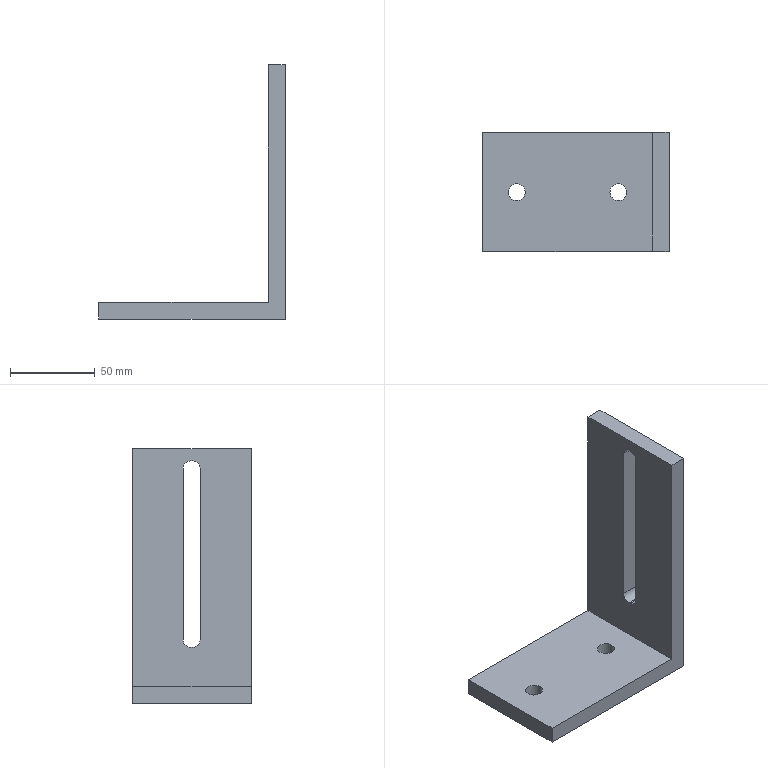Part | SolidWorks | features ICE 3, Extrusion 1 | 1 solid | 20 faces | box 110 x 70 x 150 mm | volume 162603 mm3 | plane 12 | cylinder 8 | commonest cylinder face diameters 9 x4 10 x4
STEP:
#1=CARTESIAN_POINT('',(25.,0.,0.));
#2=VERTEX_POINT('',#1);
#3=CARTESIAN_POINT('',(35.,0.,0.));
#4=VERTEX_POINT('',#3);
#5=CARTESIAN_POINT('',(30.,0.,0.));
#6=DIRECTION('',(0.,0.,1.));
#7=DIRECTION('',(1.,0.,0.));
#8=AXIS2_PLACEMENT_3D('',#5,#6,#7);
#9=CIRCLE('',#8,5.);
#10=EDGE_CURVE('',#2,#4,#9,.T.);
#11=ORIENTED_EDGE('',*,*,#10,.F.);
#12=CARTESIAN_POINT('',(25.,0.,10.));
#13=VERTEX_POINT('',#12);
#14=CARTESIAN_POINT('',(25.,0.,0.));
#15=DIRECTION('',(0.,0.,1.));
#16=VECTOR('',#15,1000.);
#17=LINE('',#14,#16);
#18=EDGE_CURVE('',#2,#13,#17,.T.);
#19=ORIENTED_EDGE('',*,*,#18,.T.);
#20=CARTESIAN_POINT('',(35.,0.,10.));
#21=VERTEX_POINT('',#20);
#22=CARTESIAN_POINT('',(30.,0.,10.));
#23=DIRECTION('',(0.,0.,1.));
#24=DIRECTION('',(1.,0.,0.));
#25=AXIS2_PLACEMENT_3D('',#22,#23,#24);
#26=CIRCLE('',#25,5.);
#27=EDGE_CURVE('',#13,#21,#26,.T.);
#28=ORIENTED_EDGE('',*,*,#27,.T.);
#29=CARTESIAN_POINT('',(35.,0.,0.));
#30=DIRECTION('',(0.,0.,1.));
#31=VECTOR('',#30,1000.);
#32=LINE('',#29,#31);
#33=EDGE_CURVE('',#4,#21,#32,.T.);
#34=ORIENTED_EDGE('',*,*,#33,.F.);
#35=EDGE_LOOP('',(#11,#19,#28,#34));
#36=FACE_OUTER_BOUND('',#35,.T.);
#37=CARTESIAN_POINT('',(30.,0.,0.));
#38=DIRECTION('',(0.,0.,1.));
#39=DIRECTION('',(1.,0.,0.));
#40=AXIS2_PLACEMENT_3D('',#37,#38,#39);
#41=CYLINDRICAL_SURFACE('',#40,5.);
#42=ADVANCED_FACE('',(#36),#41,.F.);
#43=CARTESIAN_POINT('',(-35.,0.,0.));
#44=VERTEX_POINT('',#43);
#45=CARTESIAN_POINT('',(-25.,0.,0.));
#46=VERTEX_POINT('',#45);
#47=CARTESIAN_POINT('',(-30.,0.,0.));
#48=DIRECTION('',(0.,0.,1.));
#49=DIRECTION('',(1.,0.,0.));
#50=AXIS2_PLACEMENT_3D('',#47,#48,#49);
#51=CIRCLE('',#50,5.);
#52=EDGE_CURVE('',#44,#46,#51,.T.);
#53=ORIENTED_EDGE('',*,*,#52,.F.);
#54=CARTESIAN_POINT('',(-35.,0.,10.));
#55=VERTEX_POINT('',#54);
#56=CARTESIAN_POINT('',(-35.,0.,0.));
#57=DIRECTION('',(0.,0.,1.));
#58=VECTOR('',#57,1000.);
#59=LINE('',#56,#58);
#60=EDGE_CURVE('',#44,#55,#59,.T.);
#61=ORIENTED_EDGE('',*,*,#60,.T.);
#62=CARTESIAN_POINT('',(-25.,0.,10.));
#63=VERTEX_POINT('',#62);
#64=CARTESIAN_POINT('',(-30.,0.,10.));
#65=DIRECTION('',(0.,0.,1.));
#66=DIRECTION('',(1.,0.,0.));
#67=AXIS2_PLACEMENT_3D('',#64,#65,#66);
#68=CIRCLE('',#67,5.);
#69=EDGE_CURVE('',#55,#63,#68,.T.);
#70=ORIENTED_EDGE('',*,*,#69,.T.);
#71=CARTESIAN_POINT('',(-25.,0.,0.));
#72=DIRECTION('',(0.,0.,1.));
#73=VECTOR('',#72,1000.);
#74=LINE('',#71,#73);
#75=EDGE_CURVE('',#46,#63,#74,.T.);
#76=ORIENTED_EDGE('',*,*,#75,.F.);
#77=EDGE_LOOP('',(#53,#61,#70,#76));
#78=FACE_OUTER_BOUND('',#77,.T.);
#79=CARTESIAN_POINT('',(-30.,0.,0.));
#80=DIRECTION('',(0.,0.,1.));
#81=DIRECTION('',(1.,0.,0.));
#82=AXIS2_PLACEMENT_3D('',#79,#80,#81);
#83=CYLINDRICAL_SURFACE('',#82,5.);
#84=ADVANCED_FACE('',(#78),#83,.F.);
#85=CARTESIAN_POINT('',(-50.,35.,0.));
#86=VERTEX_POINT('',#85);
#87=CARTESIAN_POINT('',(-50.,-35.,0.));
#88=VERTEX_POINT('',#87);
#89=CARTESIAN_POINT('',(-50.,-35.,0.));
#90=DIRECTION('',(0.,-1.,0.));
#91=VECTOR('',#90,1000.);
#92=LINE('',#89,#91);
#93=EDGE_CURVE('',#86,#88,#92,.T.);
#94=ORIENTED_EDGE('',*,*,#93,.T.);
#95=CARTESIAN_POINT('',(-50.,-35.,10.));
#96=VERTEX_POINT('',#95);
#97=CARTESIAN_POINT('',(-50.,-35.,10.));
#98=DIRECTION('',(0.,0.,-1.));
#99=VECTOR('',#98,1000.);
#100=LINE('',#97,#99);
#101=EDGE_CURVE('',#96,#88,#100,.T.);
#102=ORIENTED_EDGE('',*,*,#101,.F.);
#103=CARTESIAN_POINT('',(-50.,35.,10.));
#104=VERTEX_POINT('',#103);
#105=CARTESIAN_POINT('',(-50.,-35.,10.));
#106=DIRECTION('',(0.,-1.,0.));
#107=VECTOR('',#106,1000.);
#108=LINE('',#105,#107);
#109=EDGE_CURVE('',#104,#96,#108,.T.);
#110=ORIENTED_EDGE('',*,*,#109,.F.);
#111=CARTESIAN_POINT('',(-50.,35.,10.));
#112=DIRECTION('',(0.,0.,-1.));
#113=VECTOR('',#112,1000.);
#114=LINE('',#111,#113);
#115=EDGE_CURVE('',#104,#86,#114,.T.);
#116=ORIENTED_EDGE('',*,*,#115,.T.);
#117=EDGE_LOOP('',(#94,#102,#110,#116));
#118=FACE_OUTER_BOUND('',#117,.T.);
#119=CARTESIAN_POINT('',(-50.,-35.,10.));
#120=DIRECTION('',(1.,0.,0.));
#121=DIRECTION('',(0.,0.,-1.));
#122=AXIS2_PLACEMENT_3D('',#119,#120,#121);
#123=PLANE('',#122);
#124=ADVANCED_FACE('',(#118),#123,.F.);
#125=CARTESIAN_POINT('',(60.,-35.,0.));
#126=VERTEX_POINT('',#125);
#127=CARTESIAN_POINT('',(50.,-35.,0.));
#128=DIRECTION('',(1.,0.,0.));
#129=VECTOR('',#128,1000.);
#130=LINE('',#127,#129);
#131=EDGE_CURVE('',#88,#126,#130,.T.);
#132=ORIENTED_EDGE('',*,*,#131,.T.);
#133=CARTESIAN_POINT('',(60.,-35.,150.));
#134=VERTEX_POINT('',#133);
#135=CARTESIAN_POINT('',(60.,-35.,0.));
#136=DIRECTION('',(0.,0.,-1.));
#137=VECTOR('',#136,1000.);
#138=LINE('',#135,#137);
#139=EDGE_CURVE('',#134,#126,#138,.T.);
#140=ORIENTED_EDGE('',*,*,#139,.F.);
#141=CARTESIAN_POINT('',(50.,-35.,150.));
#142=VERTEX_POINT('',#141);
#143=CARTESIAN_POINT('',(60.,-35.,150.));
#144=DIRECTION('',(-1.,0.,0.));
#145=VECTOR('',#144,1000.);
#146=LINE('',#143,#145);
#147=EDGE_CURVE('',#134,#142,#146,.T.);
#148=ORIENTED_EDGE('',*,*,#147,.T.);
#149=CARTESIAN_POINT('',(50.,-35.,10.));
#150=VERTEX_POINT('',#149);
#151=CARTESIAN_POINT('',(50.,-35.,0.));
#152=DIRECTION('',(0.,0.,-1.));
#153=VECTOR('',#152,1000.);
#154=LINE('',#151,#153);
#155=EDGE_CURVE('',#142,#150,#154,.T.);
#156=ORIENTED_EDGE('',*,*,#155,.T.);
#157=CARTESIAN_POINT('',(50.,-35.,10.));
#158=DIRECTION('',(1.,0.,0.));
#159=VECTOR('',#158,1000.);
#160=LINE('',#157,#159);
#161=EDGE_CURVE('',#96,#150,#160,.T.);
#162=ORIENTED_EDGE('',*,*,#161,.F.);
#163=ORIENTED_EDGE('',*,*,#101,.T.);
#164=EDGE_LOOP('',(#132,#140,#148,#156,#162,#163));
#165=FACE_OUTER_BOUND('',#164,.T.);
#166=CARTESIAN_POINT('',(50.,-35.,10.));
#167=DIRECTION('',(0.,1.,0.));
#168=DIRECTION('',(-1.,0.,0.));
#169=AXIS2_PLACEMENT_3D('',#166,#167,#168);
#170=PLANE('',#169);
#171=ADVANCED_FACE('',(#165),#170,.F.);
#172=CARTESIAN_POINT('',(60.,35.,0.));
#173=VERTEX_POINT('',#172);
#174=CARTESIAN_POINT('',(50.,35.,0.));
#175=DIRECTION('',(-1.,0.,0.));
#176=VECTOR('',#175,1000.);
#177=LINE('',#174,#176);
#178=EDGE_CURVE('',#173,#86,#177,.T.);
#179=ORIENTED_EDGE('',*,*,#178,.T.);
#180=ORIENTED_EDGE('',*,*,#115,.F.);
#181=CARTESIAN_POINT('',(50.,35.,10.));
#182=VERTEX_POINT('',#181);
#183=CARTESIAN_POINT('',(50.,35.,10.));
#184=DIRECTION('',(-1.,0.,0.));
#185=VECTOR('',#184,1000.);
#186=LINE('',#183,#185);
#187=EDGE_CURVE('',#182,#104,#186,.T.);
#188=ORIENTED_EDGE('',*,*,#187,.F.);
#189=CARTESIAN_POINT('',(50.,35.,150.));
#190=VERTEX_POINT('',#189);
#191=CARTESIAN_POINT('',(50.,35.,0.));
#192=DIRECTION('',(0.,0.,1.));
#193=VECTOR('',#192,1000.);
#194=LINE('',#191,#193);
#195=EDGE_CURVE('',#182,#190,#194,.T.);
#196=ORIENTED_EDGE('',*,*,#195,.T.);
#197=CARTESIAN_POINT('',(60.,35.,150.));
#198=VERTEX_POINT('',#197);
#199=CARTESIAN_POINT('',(60.,35.,150.));
#200=DIRECTION('',(-1.,0.,0.));
#201=VECTOR('',#200,1000.);
#202=LINE('',#199,#201);
#203=EDGE_CURVE('',#198,#190,#202,.T.);
#204=ORIENTED_EDGE('',*,*,#203,.F.);
#205=CARTESIAN_POINT('',(60.,35.,0.));
#206=DIRECTION('',(0.,0.,1.));
#207=VECTOR('',#206,1000.);
#208=LINE('',#205,#207);
#209=EDGE_CURVE('',#173,#198,#208,.T.);
#210=ORIENTED_EDGE('',*,*,#209,.F.);
#211=EDGE_LOOP('',(#179,#180,#188,#196,#204,#210));
#212=FACE_OUTER_BOUND('',#211,.T.);
#213=CARTESIAN_POINT('',(50.,35.,10.));
#214=DIRECTION('',(0.,-1.,0.));
#215=DIRECTION('',(1.,0.,0.));
#216=AXIS2_PLACEMENT_3D('',#213,#214,#215);
#217=PLANE('',#216);
#218=ADVANCED_FACE('',(#212),#217,.F.);
#219=CARTESIAN_POINT('',(30.,0.,10.));
#220=DIRECTION('',(0.,0.,1.));
#221=DIRECTION('',(1.,0.,0.));
#222=AXIS2_PLACEMENT_3D('',#219,#220,#221);
#223=CIRCLE('',#222,5.);
#224=EDGE_CURVE('',#21,#13,#223,.T.);
#225=ORIENTED_EDGE('',*,*,#224,.F.);
#226=ORIENTED_EDGE('',*,*,#27,.F.);
#227=EDGE_LOOP('',(#225,#226));
#228=FACE_BOUND('',#227,.T.);
#229=CARTESIAN_POINT('',(-30.,0.,10.));
#230=DIRECTION('',(0.,0.,1.));
#231=DIRECTION('',(1.,0.,0.));
#232=AXIS2_PLACEMENT_3D('',#229,#230,#231);
#233=CIRCLE('',#232,5.);
#234=EDGE_CURVE('',#63,#55,#233,.T.);
#235=ORIENTED_EDGE('',*,*,#234,.F.);
#236=ORIENTED_EDGE('',*,*,#69,.F.);
#237=EDGE_LOOP('',(#235,#236));
#238=FACE_BOUND('',#237,.T.);
#239=ORIENTED_EDGE('',*,*,#109,.T.);
#240=ORIENTED_EDGE('',*,*,#161,.T.);
#241=CARTESIAN_POINT('',(50.,-35.,10.));
#242=DIRECTION('',(0.,1.,0.));
#243=VECTOR('',#242,1000.);
#244=LINE('',#241,#243);
#245=EDGE_CURVE('',#150,#182,#244,.T.);
#246=ORIENTED_EDGE('',*,*,#245,.T.);
#247=ORIENTED_EDGE('',*,*,#187,.T.);
#248=EDGE_LOOP('',(#239,#240,#246,#247));
#249=FACE_OUTER_BOUND('',#248,.T.);
#250=CARTESIAN_POINT('',(-50.,35.,10.));
#251=DIRECTION('',(0.,0.,1.));
#252=DIRECTION('',(1.,0.,0.));
#253=AXIS2_PLACEMENT_3D('',#250,#251,#252);
#254=PLANE('',#253);
#255=ADVANCED_FACE('',(#228,#238,#249),#254,.T.);
#256=CARTESIAN_POINT('',(30.,0.,0.));
#257=DIRECTION('',(0.,0.,1.));
#258=DIRECTION('',(1.,0.,0.));
#259=AXIS2_PLACEMENT_3D('',#256,#257,#258);
#260=CIRCLE('',#259,5.);
#261=EDGE_CURVE('',#4,#2,#260,.T.);
#262=ORIENTED_EDGE('',*,*,#261,.T.);
#263=ORIENTED_EDGE('',*,*,#10,.T.);
#264=EDGE_LOOP('',(#262,#263));
#265=FACE_BOUND('',#264,.T.);
#266=CARTESIAN_POINT('',(-30.,0.,0.));
#267=DIRECTION('',(0.,0.,1.));
#268=DIRECTION('',(1.,0.,0.));
#269=AXIS2_PLACEMENT_3D('',#266,#267,#268);
#270=CIRCLE('',#269,5.);
#271=EDGE_CURVE('',#46,#44,#270,.T.);
#272=ORIENTED_EDGE('',*,*,#271,.T.);
#273=ORIENTED_EDGE('',*,*,#52,.T.);
#274=EDGE_LOOP('',(#272,#273));
#275=FACE_BOUND('',#274,.T.);
#276=ORIENTED_EDGE('',*,*,#93,.F.);
#277=ORIENTED_EDGE('',*,*,#178,.F.);
#278=CARTESIAN_POINT('',(60.,35.,0.));
#279=DIRECTION('',(0.,1.,0.));
#280=VECTOR('',#279,1000.);
#281=LINE('',#278,#280);
#282=EDGE_CURVE('',#126,#173,#281,.T.);
#283=ORIENTED_EDGE('',*,*,#282,.F.);
#284=ORIENTED_EDGE('',*,*,#131,.F.);
#285=EDGE_LOOP('',(#276,#277,#283,#284));
#286=FACE_OUTER_BOUND('',#285,.T.);
#287=CARTESIAN_POINT('',(-50.,35.,0.));
#288=DIRECTION('',(0.,0.,1.));
#289=DIRECTION('',(1.,0.,0.));
#290=AXIS2_PLACEMENT_3D('',#287,#288,#289);
#291=PLANE('',#290);
#292=ADVANCED_FACE('',(#265,#275,#286),#291,.F.);
#293=ORIENTED_EDGE('',*,*,#60,.F.);
#294=ORIENTED_EDGE('',*,*,#271,.F.);
#295=ORIENTED_EDGE('',*,*,#75,.T.);
#296=ORIENTED_EDGE('',*,*,#234,.T.);
#297=EDGE_LOOP('',(#293,#294,#295,#296));
#298=FACE_OUTER_BOUND('',#297,.T.);
#299=CARTESIAN_POINT('',(-30.,0.,0.));
#300=DIRECTION('',(0.,0.,1.));
#301=DIRECTION('',(1.,0.,0.));
#302=AXIS2_PLACEMENT_3D('',#299,#300,#301);
#303=CYLINDRICAL_SURFACE('',#302,5.);
#304=ADVANCED_FACE('',(#298),#303,.F.);
#305=ORIENTED_EDGE('',*,*,#18,.F.);
#306=ORIENTED_EDGE('',*,*,#261,.F.);
#307=ORIENTED_EDGE('',*,*,#33,.T.);
#308=ORIENTED_EDGE('',*,*,#224,.T.);
#309=EDGE_LOOP('',(#305,#306,#307,#308));
#310=FACE_OUTER_BOUND('',#309,.T.);
#311=CARTESIAN_POINT('',(30.,0.,0.));
#312=DIRECTION('',(0.,0.,1.));
#313=DIRECTION('',(1.,0.,0.));
#314=AXIS2_PLACEMENT_3D('',#311,#312,#313);
#315=CYLINDRICAL_SURFACE('',#314,5.);
#316=ADVANCED_FACE('',(#310),#315,.F.);
#317=CARTESIAN_POINT('',(50.,0.7048,142.896));
#318=VERTEX_POINT('',#317);
#319=CARTESIAN_POINT('',(50.,5.205,138.396));
#320=VERTEX_POINT('',#319);
#321=CARTESIAN_POINT('',(50.,0.7048,138.396));
#322=DIRECTION('',(-1.,0.,0.));
#323=DIRECTION('',(0.,0.,1.));
#324=AXIS2_PLACEMENT_3D('',#321,#322,#323);
#325=CIRCLE('',#324,4.5);
#326=EDGE_CURVE('',#318,#320,#325,.T.);
#327=ORIENTED_EDGE('',*,*,#326,.F.);
#328=CARTESIAN_POINT('',(50.,-0.2952,142.896));
#329=VERTEX_POINT('',#328);
#330=CARTESIAN_POINT('',(50.,-0.2952,142.896));
#331=DIRECTION('',(0.,1.,0.));
#332=VECTOR('',#331,1000.);
#333=LINE('',#330,#332);
#334=EDGE_CURVE('',#329,#318,#333,.T.);
#335=ORIENTED_EDGE('',*,*,#334,.F.);
#336=CARTESIAN_POINT('',(50.,-4.795,138.396));
#337=VERTEX_POINT('',#336);
#338=CARTESIAN_POINT('',(50.,-0.2952,138.396));
#339=DIRECTION('',(-1.,0.,0.));
#340=DIRECTION('',(0.,0.,1.));
#341=AXIS2_PLACEMENT_3D('',#338,#339,#340);
#342=CIRCLE('',#341,4.5);
#343=EDGE_CURVE('',#337,#329,#342,.T.);
#344=ORIENTED_EDGE('',*,*,#343,.F.);
#345=CARTESIAN_POINT('',(50.,-4.795,37.396));
#346=VERTEX_POINT('',#345);
#347=CARTESIAN_POINT('',(50.,-4.795,138.396));
#348=DIRECTION('',(0.,0.,1.));
#349=VECTOR('',#348,1000.);
#350=LINE('',#347,#349);
#351=EDGE_CURVE('',#346,#337,#350,.T.);
#352=ORIENTED_EDGE('',*,*,#351,.F.);
#353=CARTESIAN_POINT('',(50.,-0.2952,32.896));
#354=VERTEX_POINT('',#353);
#355=CARTESIAN_POINT('',(50.,-0.2952,37.396));
#356=DIRECTION('',(-1.,0.,0.));
#357=DIRECTION('',(0.,0.,-1.));
#358=AXIS2_PLACEMENT_3D('',#355,#356,#357);
#359=CIRCLE('',#358,4.5);
#360=EDGE_CURVE('',#354,#346,#359,.T.);
#361=ORIENTED_EDGE('',*,*,#360,.F.);
#362=CARTESIAN_POINT('',(50.,0.7048,32.896));
#363=VERTEX_POINT('',#362);
#364=CARTESIAN_POINT('',(50.,-0.2952,32.896));
#365=DIRECTION('',(0.,-1.,0.));
#366=VECTOR('',#365,1000.);
#367=LINE('',#364,#366);
#368=EDGE_CURVE('',#363,#354,#367,.T.);
#369=ORIENTED_EDGE('',*,*,#368,.F.);
#370=CARTESIAN_POINT('',(50.,5.205,37.396));
#371=VERTEX_POINT('',#370);
#372=CARTESIAN_POINT('',(50.,0.7048,37.396));
#373=DIRECTION('',(-1.,0.,0.));
#374=DIRECTION('',(0.,0.,1.));
#375=AXIS2_PLACEMENT_3D('',#372,#373,#374);
#376=CIRCLE('',#375,4.5);
#377=EDGE_CURVE('',#371,#363,#376,.T.);
#378=ORIENTED_EDGE('',*,*,#377,.F.);
#379=CARTESIAN_POINT('',(50.,5.205,138.396));
#380=DIRECTION('',(0.,0.,-1.));
#381=VECTOR('',#380,1000.);
#382=LINE('',#379,#381);
#383=EDGE_CURVE('',#320,#371,#382,.T.);
#384=ORIENTED_EDGE('',*,*,#383,.F.);
#385=EDGE_LOOP('',(#327,#335,#344,#352,#361,#369,#378,#384));
#386=FACE_BOUND('',#385,.T.);
#387=ORIENTED_EDGE('',*,*,#245,.F.);
#388=ORIENTED_EDGE('',*,*,#155,.F.);
#389=CARTESIAN_POINT('',(50.,35.,150.));
#390=DIRECTION('',(0.,-1.,0.));
#391=VECTOR('',#390,1000.);
#392=LINE('',#389,#391);
#393=EDGE_CURVE('',#190,#142,#392,.T.);
#394=ORIENTED_EDGE('',*,*,#393,.F.);
#395=ORIENTED_EDGE('',*,*,#195,.F.);
#396=EDGE_LOOP('',(#387,#388,#394,#395));
#397=FACE_OUTER_BOUND('',#396,.T.);
#398=CARTESIAN_POINT('',(50.,-35.,0.));
#399=DIRECTION('',(-1.,0.,0.));
#400=DIRECTION('',(0.,0.,1.));
#401=AXIS2_PLACEMENT_3D('',#398,#399,#400);
#402=PLANE('',#401);
#403=ADVANCED_FACE('',(#386,#397),#402,.T.);
#404=ORIENTED_EDGE('',*,*,#393,.T.);
#405=ORIENTED_EDGE('',*,*,#147,.F.);
#406=CARTESIAN_POINT('',(60.,35.,150.));
#407=DIRECTION('',(0.,-1.,0.));
#408=VECTOR('',#407,1000.);
#409=LINE('',#406,#408);
#410=EDGE_CURVE('',#198,#134,#409,.T.);
#411=ORIENTED_EDGE('',*,*,#410,.F.);
#412=ORIENTED_EDGE('',*,*,#203,.T.);
#413=EDGE_LOOP('',(#404,#405,#411,#412));
#414=FACE_OUTER_BOUND('',#413,.T.);
#415=CARTESIAN_POINT('',(60.,35.,150.));
#416=DIRECTION('',(0.,0.,-1.));
#417=DIRECTION('',(-1.,0.,0.));
#418=AXIS2_PLACEMENT_3D('',#415,#416,#417);
#419=PLANE('',#418);
#420=ADVANCED_FACE('',(#414),#419,.F.);
#421=CARTESIAN_POINT('',(60.,-0.2952,142.896));
#422=VERTEX_POINT('',#421);
#423=CARTESIAN_POINT('',(60.,0.7048,142.896));
#424=VERTEX_POINT('',#423);
#425=CARTESIAN_POINT('',(60.,-35.,142.896));
#426=DIRECTION('',(0.,1.,0.));
#427=VECTOR('',#426,1000.);
#428=LINE('',#425,#427);
#429=EDGE_CURVE('',#422,#424,#428,.T.);
#430=ORIENTED_EDGE('',*,*,#429,.T.);
#431=CARTESIAN_POINT('',(60.,5.205,138.396));
#432=VERTEX_POINT('',#431);
#433=CARTESIAN_POINT('',(60.,0.7048,138.396));
#434=DIRECTION('',(-1.,0.,0.));
#435=DIRECTION('',(0.,0.,1.));
#436=AXIS2_PLACEMENT_3D('',#433,#434,#435);
#437=CIRCLE('',#436,4.5);
#438=EDGE_CURVE('',#424,#432,#437,.T.);
#439=ORIENTED_EDGE('',*,*,#438,.T.);
#440=CARTESIAN_POINT('',(60.,5.205,37.396));
#441=VERTEX_POINT('',#440);
#442=CARTESIAN_POINT('',(60.,5.205,0.));
#443=DIRECTION('',(0.,0.,-1.));
#444=VECTOR('',#443,1000.);
#445=LINE('',#442,#444);
#446=EDGE_CURVE('',#432,#441,#445,.T.);
#447=ORIENTED_EDGE('',*,*,#446,.T.);
#448=CARTESIAN_POINT('',(60.,0.7048,32.896));
#449=VERTEX_POINT('',#448);
#450=CARTESIAN_POINT('',(60.,0.7048,37.396));
#451=DIRECTION('',(-1.,0.,0.));
#452=DIRECTION('',(0.,0.,1.));
#453=AXIS2_PLACEMENT_3D('',#450,#451,#452);
#454=CIRCLE('',#453,4.5);
#455=EDGE_CURVE('',#441,#449,#454,.T.);
#456=ORIENTED_EDGE('',*,*,#455,.T.);
#457=CARTESIAN_POINT('',(60.,-0.2952,32.896));
#458=VERTEX_POINT('',#457);
#459=CARTESIAN_POINT('',(60.,-35.,32.896));
#460=DIRECTION('',(0.,-1.,0.));
#461=VECTOR('',#460,1000.);
#462=LINE('',#459,#461);
#463=EDGE_CURVE('',#449,#458,#462,.T.);
#464=ORIENTED_EDGE('',*,*,#463,.T.);
#465=CARTESIAN_POINT('',(60.,-4.795,37.396));
#466=VERTEX_POINT('',#465);
#467=CARTESIAN_POINT('',(60.,-0.2952,37.396));
#468=DIRECTION('',(-1.,0.,0.));
#469=DIRECTION('',(0.,0.,1.));
#470=AXIS2_PLACEMENT_3D('',#467,#468,#469);
#471=CIRCLE('',#470,4.5);
#472=EDGE_CURVE('',#458,#466,#471,.T.);
#473=ORIENTED_EDGE('',*,*,#472,.T.);
#474=CARTESIAN_POINT('',(60.,-4.795,138.396));
#475=VERTEX_POINT('',#474);
#476=CARTESIAN_POINT('',(60.,-4.795,0.));
#477=DIRECTION('',(0.,0.,1.));
#478=VECTOR('',#477,1000.);
#479=LINE('',#476,#478);
#480=EDGE_CURVE('',#466,#475,#479,.T.);
#481=ORIENTED_EDGE('',*,*,#480,.T.);
#482=CARTESIAN_POINT('',(60.,-0.2952,138.396));
#483=DIRECTION('',(-1.,0.,0.));
#484=DIRECTION('',(0.,0.,1.));
#485=AXIS2_PLACEMENT_3D('',#482,#483,#484);
#486=CIRCLE('',#485,4.5);
#487=EDGE_CURVE('',#475,#422,#486,.T.);
#488=ORIENTED_EDGE('',*,*,#487,.T.);
#489=EDGE_LOOP('',(#430,#439,#447,#456,#464,#473,#481,#488));
#490=FACE_BOUND('',#489,.T.);
#491=ORIENTED_EDGE('',*,*,#282,.T.);
#492=ORIENTED_EDGE('',*,*,#209,.T.);
#493=ORIENTED_EDGE('',*,*,#410,.T.);
#494=ORIENTED_EDGE('',*,*,#139,.T.);
#495=EDGE_LOOP('',(#491,#492,#493,#494));
#496=FACE_OUTER_BOUND('',#495,.T.);
#497=CARTESIAN_POINT('',(60.,-35.,0.));
#498=DIRECTION('',(-1.,0.,0.));
#499=DIRECTION('',(0.,0.,1.));
#500=AXIS2_PLACEMENT_3D('',#497,#498,#499);
#501=PLANE('',#500);
#502=ADVANCED_FACE('',(#490,#496),#501,.F.);
#503=CARTESIAN_POINT('',(100.,0.7048,142.896));
#504=DIRECTION('',(-1.,0.,0.));
#505=VECTOR('',#504,1000.);
#506=LINE('',#503,#505);
#507=EDGE_CURVE('',#424,#318,#506,.T.);
#508=ORIENTED_EDGE('',*,*,#507,.T.);
#509=ORIENTED_EDGE('',*,*,#326,.T.);
#510=CARTESIAN_POINT('',(100.,5.205,138.396));
#511=DIRECTION('',(-1.,0.,0.));
#512=VECTOR('',#511,1000.);
#513=LINE('',#510,#512);
#514=EDGE_CURVE('',#432,#320,#513,.T.);
#515=ORIENTED_EDGE('',*,*,#514,.F.);
#516=ORIENTED_EDGE('',*,*,#438,.F.);
#517=EDGE_LOOP('',(#508,#509,#515,#516));
#518=FACE_OUTER_BOUND('',#517,.T.);
#519=CARTESIAN_POINT('',(100.,0.7048,138.396));
#520=DIRECTION('',(-1.,0.,0.));
#521=DIRECTION('',(0.,0.,1.));
#522=AXIS2_PLACEMENT_3D('',#519,#520,#521);
#523=CYLINDRICAL_SURFACE('',#522,4.5);
#524=ADVANCED_FACE('',(#518),#523,.F.);
#525=CARTESIAN_POINT('',(100.,-0.2952,142.896));
#526=DIRECTION('',(-1.,0.,0.));
#527=VECTOR('',#526,1000.);
#528=LINE('',#525,#527);
#529=EDGE_CURVE('',#422,#329,#528,.T.);
#530=ORIENTED_EDGE('',*,*,#529,.T.);
#531=ORIENTED_EDGE('',*,*,#334,.T.);
#532=ORIENTED_EDGE('',*,*,#507,.F.);
#533=ORIENTED_EDGE('',*,*,#429,.F.);
#534=EDGE_LOOP('',(#530,#531,#532,#533));
#535=FACE_OUTER_BOUND('',#534,.T.);
#536=CARTESIAN_POINT('',(100.,-0.2952,142.896));
#537=DIRECTION('',(0.,0.,1.));
#538=DIRECTION('',(1.,0.,0.));
#539=AXIS2_PLACEMENT_3D('',#536,#537,#538);
#540=PLANE('',#539);
#541=ADVANCED_FACE('',(#535),#540,.F.);
#542=CARTESIAN_POINT('',(100.,-4.795,138.396));
#543=DIRECTION('',(-1.,0.,0.));
#544=VECTOR('',#543,1000.);
#545=LINE('',#542,#544);
#546=EDGE_CURVE('',#475,#337,#545,.T.);
#547=ORIENTED_EDGE('',*,*,#546,.T.);
#548=ORIENTED_EDGE('',*,*,#343,.T.);
#549=ORIENTED_EDGE('',*,*,#529,.F.);
#550=ORIENTED_EDGE('',*,*,#487,.F.);
#551=EDGE_LOOP('',(#547,#548,#549,#550));
#552=FACE_OUTER_BOUND('',#551,.T.);
#553=CARTESIAN_POINT('',(100.,-0.2952,138.396));
#554=DIRECTION('',(-1.,0.,0.));
#555=DIRECTION('',(0.,0.,1.));
#556=AXIS2_PLACEMENT_3D('',#553,#554,#555);
#557=CYLINDRICAL_SURFACE('',#556,4.5);
#558=ADVANCED_FACE('',(#552),#557,.F.);
#559=CARTESIAN_POINT('',(100.,-4.795,37.396));
#560=DIRECTION('',(-1.,0.,0.));
#561=VECTOR('',#560,1000.);
#562=LINE('',#559,#561);
#563=EDGE_CURVE('',#466,#346,#562,.T.);
#564=ORIENTED_EDGE('',*,*,#563,.T.);
#565=ORIENTED_EDGE('',*,*,#351,.T.);
#566=ORIENTED_EDGE('',*,*,#546,.F.);
#567=ORIENTED_EDGE('',*,*,#480,.F.);
#568=EDGE_LOOP('',(#564,#565,#566,#567));
#569=FACE_OUTER_BOUND('',#568,.T.);
#570=CARTESIAN_POINT('',(100.,-4.795,138.396));
#571=DIRECTION('',(0.,-1.,0.));
#572=DIRECTION('',(0.,0.,-1.));
#573=AXIS2_PLACEMENT_3D('',#570,#571,#572);
#574=PLANE('',#573);
#575=ADVANCED_FACE('',(#569),#574,.F.);
#576=CARTESIAN_POINT('',(100.,-0.2952,32.896));
#577=DIRECTION('',(-1.,0.,0.));
#578=VECTOR('',#577,1000.);
#579=LINE('',#576,#578);
#580=EDGE_CURVE('',#458,#354,#579,.T.);
#581=ORIENTED_EDGE('',*,*,#580,.T.);
#582=ORIENTED_EDGE('',*,*,#360,.T.);
#583=ORIENTED_EDGE('',*,*,#563,.F.);
#584=ORIENTED_EDGE('',*,*,#472,.F.);
#585=EDGE_LOOP('',(#581,#582,#583,#584));
#586=FACE_OUTER_BOUND('',#585,.T.);
#587=CARTESIAN_POINT('',(100.,-0.2952,37.396));
#588=DIRECTION('',(-1.,0.,0.));
#589=DIRECTION('',(0.,0.,1.));
#590=AXIS2_PLACEMENT_3D('',#587,#588,#589);
#591=CYLINDRICAL_SURFACE('',#590,4.5);
#592=ADVANCED_FACE('',(#586),#591,.F.);
#593=CARTESIAN_POINT('',(100.,0.7048,32.896));
#594=DIRECTION('',(-1.,0.,0.));
#595=VECTOR('',#594,1000.);
#596=LINE('',#593,#595);
#597=EDGE_CURVE('',#449,#363,#596,.T.);
#598=ORIENTED_EDGE('',*,*,#597,.T.);
#599=ORIENTED_EDGE('',*,*,#368,.T.);
#600=ORIENTED_EDGE('',*,*,#580,.F.);
#601=ORIENTED_EDGE('',*,*,#463,.F.);
#602=EDGE_LOOP('',(#598,#599,#600,#601));
#603=FACE_OUTER_BOUND('',#602,.T.);
#604=CARTESIAN_POINT('',(100.,-0.2952,32.896));
#605=DIRECTION('',(0.,0.,-1.));
#606=DIRECTION('',(-1.,0.,0.));
#607=AXIS2_PLACEMENT_3D('',#604,#605,#606);
#608=PLANE('',#607);
#609=ADVANCED_FACE('',(#603),#608,.F.);
#610=CARTESIAN_POINT('',(100.,5.205,37.396));
#611=DIRECTION('',(-1.,0.,0.));
#612=VECTOR('',#611,1000.);
#613=LINE('',#610,#612);
#614=EDGE_CURVE('',#441,#371,#613,.T.);
#615=ORIENTED_EDGE('',*,*,#614,.T.);
#616=ORIENTED_EDGE('',*,*,#377,.T.);
#617=ORIENTED_EDGE('',*,*,#597,.F.);
#618=ORIENTED_EDGE('',*,*,#455,.F.);
#619=EDGE_LOOP('',(#615,#616,#617,#618));
#620=FACE_OUTER_BOUND('',#619,.T.);
#621=CARTESIAN_POINT('',(100.,0.7048,37.396));
#622=DIRECTION('',(-1.,0.,0.));
#623=DIRECTION('',(0.,0.,1.));
#624=AXIS2_PLACEMENT_3D('',#621,#622,#623);
#625=CYLINDRICAL_SURFACE('',#624,4.5);
#626=ADVANCED_FACE('',(#620),#625,.F.);
#627=ORIENTED_EDGE('',*,*,#514,.T.);
#628=ORIENTED_EDGE('',*,*,#383,.T.);
#629=ORIENTED_EDGE('',*,*,#614,.F.);
#630=ORIENTED_EDGE('',*,*,#446,.F.);
#631=EDGE_LOOP('',(#627,#628,#629,#630));
#632=FACE_OUTER_BOUND('',#631,.T.);
#633=CARTESIAN_POINT('',(100.,5.205,138.396));
#634=DIRECTION('',(0.,1.,0.));
#635=DIRECTION('',(0.,0.,1.));
#636=AXIS2_PLACEMENT_3D('',#633,#634,#635);
#637=PLANE('',#636);
#638=ADVANCED_FACE('',(#632),#637,.F.);
#639=CLOSED_SHELL('',(#42,#84,#124,#171,#218,#255,#292,#304,#316,#403,#420,#502,#524,#541,#558,#575,#592,#609,#626,#638));
#640=MANIFOLD_SOLID_BREP('',#639);
#641=CARTESIAN_POINT('',(0.,0.,0.));
#642=DIRECTION('',(0.,0.,1.));
#643=DIRECTION('',(1.,0.,0.));
#644=AXIS2_PLACEMENT_3D('',#641,#642,#643);
#645=(LENGTH_UNIT()NAMED_UNIT(*)SI_UNIT(.MILLI.,.METRE.));
#646=UNCERTAINTY_MEASURE_WITH_UNIT(LENGTH_MEASURE(0.00001),#645,'','');
#647=(NAMED_UNIT(*)PLANE_ANGLE_UNIT()SI_UNIT($,.RADIAN.));
#648=(NAMED_UNIT(*)SI_UNIT($,.STERADIAN.)SOLID_ANGLE_UNIT());
#649=(GEOMETRIC_REPRESENTATION_CONTEXT(3)GLOBAL_UNCERTAINTY_ASSIGNED_CONTEXT((#646))GLOBAL_UNIT_ASSIGNED_CONTEXT((#645,#647,#648))REPRESENTATION_CONTEXT('',''));
#650=ADVANCED_BREP_SHAPE_REPRESENTATION('',(#640,#644),#649);